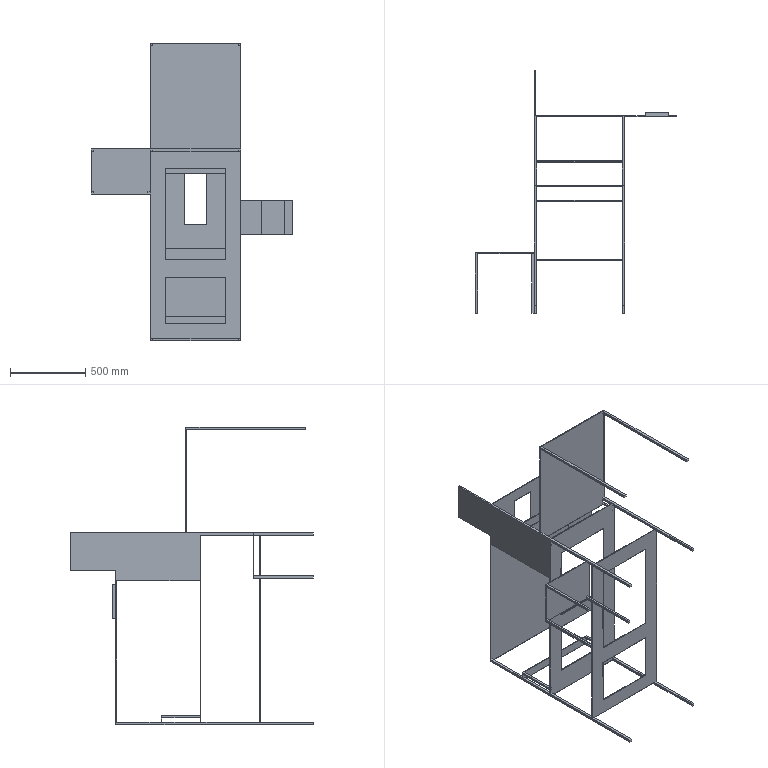Part | SolidWorks | features ICE 26, MirrorPattern 3, Cut 1, Extrusion 1, LPattern 1 | 1 solid | 125 faces | box 1333 x 1609 x 1972 mm | volume 16595563 mm3 | plane 125